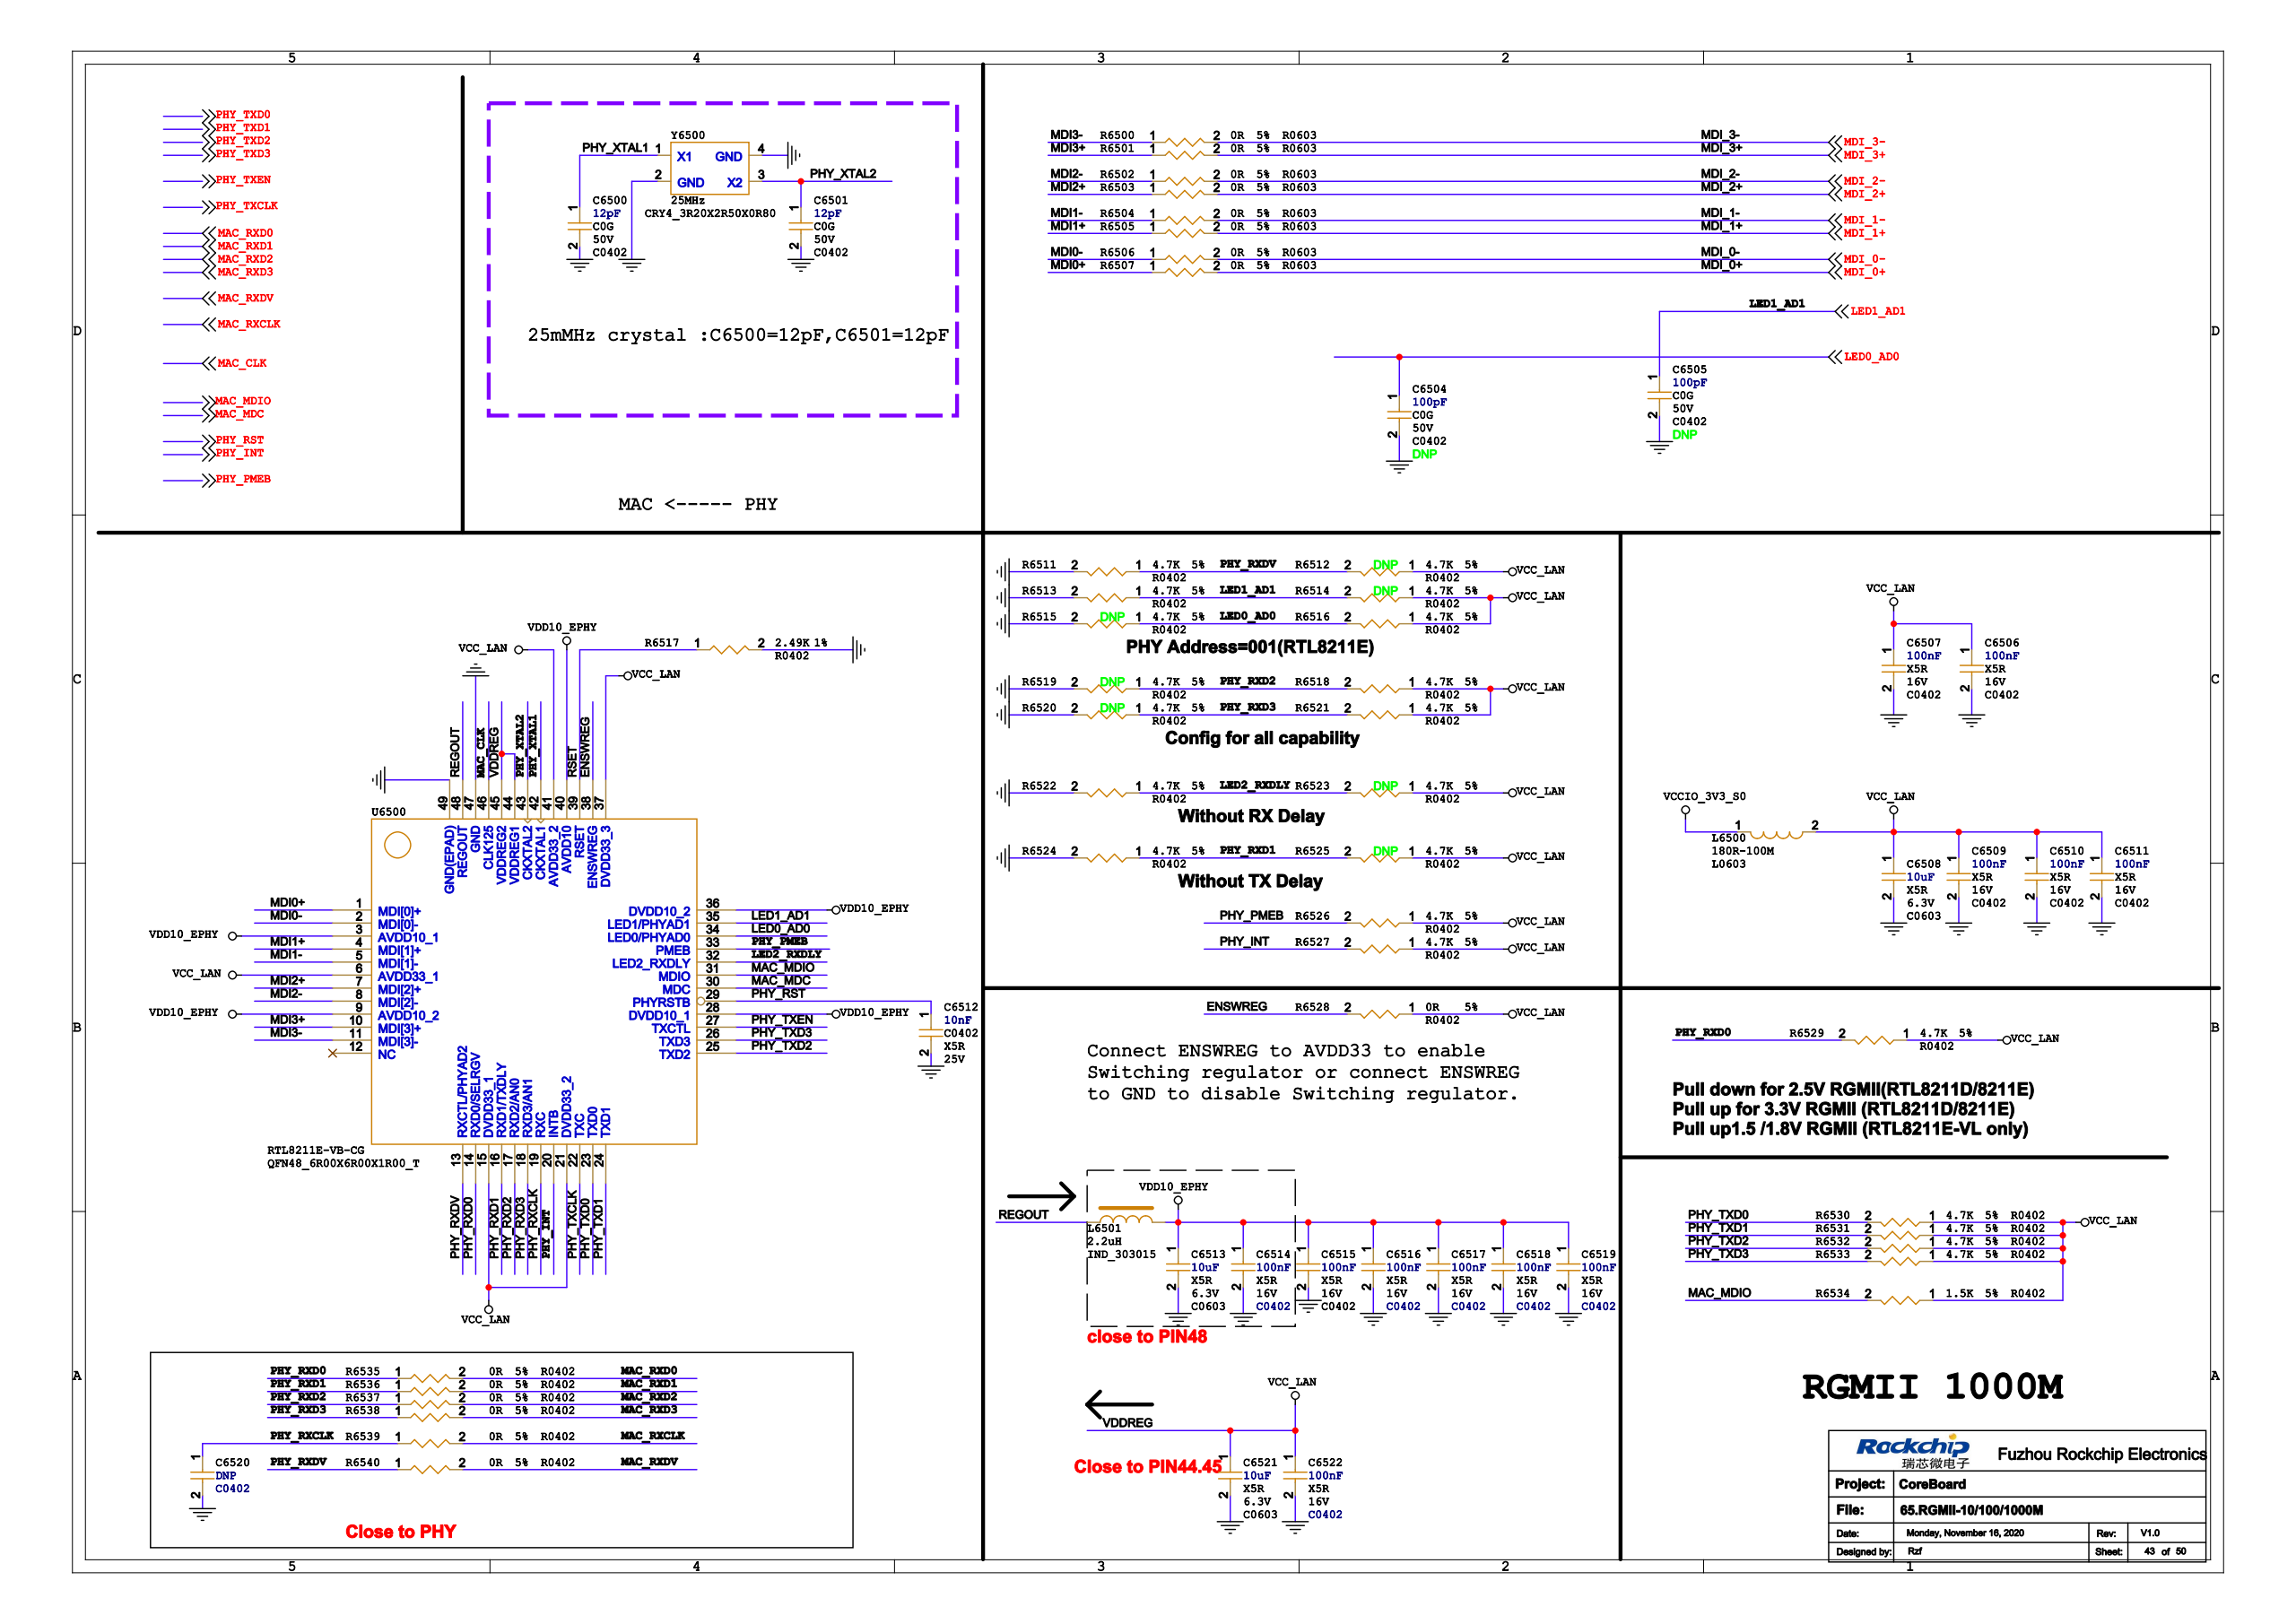Circuit board | Cadence Allegro | 749 parts | 717 nets | one sheet of the schematic
Parts on this sheet (reference | value | footprint):
C6500 | 12pF | C0402
C6501 | 12pF | C0402
C6504 | 100pF | C0402
C6505 | 100pF | C0402
C6506 | 100nF | C0402
C6507 | 100nF | C0402
C6508 | 10uF | C0603
C6509 | 100nF | C0402
C6510 | 100nF | C0402
C6511 | 100nF | C0402
C6512 | 10nF | C0402
C6513 | 10uF | C0603
C6514 | 100nF | C0402
C6515 | 100nF | C0402
C6516 | 100nF | C0402
C6517 | 100nF | C0402
C6518 | 100nF | C0402
C6519 | 100nF | C0402
C6520 | DNP | C0402
C6521 | 10uF | C0603
C6522 | 100nF | C0402
L6500 | 180R-100M | L0603
L6501 | 2.2uH | IND_303015
R6500 | 0R | R0603
R6501 | 0R | R0603
R6502 | 0R | R0603
R6503 | 0R | R0603
R6504 | 0R | R0603
R6505 | 0R | R0603
R6506 | 0R | R0603
R6507 | 0R | R0603
R6511 | 4.7K | R0402
R6512 | 4.7K | R0402
R6513 | 4.7K | R0402
R6514 | 4.7K | R0402
R6515 | 4.7K | R0402
R6516 | 4.7K | R0402
R6517 | 2.49K | R0402
R6518 | 4.7K | R0402
R6519 | 4.7K | R0402
R6520 | 4.7K | R0402
R6521 | 4.7K | R0402
R6522 | 4.7K | R0402
R6523 | 4.7K | R0402
R6524 | 4.7K | R0402
R6525 | 4.7K | R0402
R6526 | 4.7K | R0402
R6527 | 4.7K | R0402
R6528 | 0R | R0402
R6529 | 4.7K | R0402
R6530 | 4.7K | R0402
R6531 | 4.7K | R0402
R6532 | 4.7K | R0402
R6533 | 4.7K | R0402
R6534 | 1.5K | R0402
R6535 | 0R | R0402
R6536 | 0R | R0402
R6537 | 0R | R0402
R6538 | 0R | R0402
R6539 | 0R | R0402
R6540 | 0R | R0402
U6500 | RTL8211E-VB-CG | QFN48_6R00X6R00X1R00_T
Y6500 | 25MHz | CRY4_3R20X2R50X0R80
Nets of these parts (net: part-pin ...):
GND: C6500-2 C6501-2 C6504-2 C6505-2 C6506-2 C6507-2 C6508-2 C6509-2 C6510-2 C6511-2 C6512-2 C6513-2 C6514-2 C6515-2 C6516-2 C6517-2 C6518-2 C6519-2 C6520-2 C6521-2 C6522-2 R6511-2 R6513-2 R6515-2 R6517-2 R6519-2 R6520-2 R6522-2 R6524-2 Y6500-2 Y6500-4 U6500-47 U6500-49
PHY_XTAL1: C6500-1 Y6500-1 U6500-42
PHY_XTAL2: C6501-1 Y6500-3 U6500-43
PHY_RST: C6512-1 U6500-29
LED0_AD0: C6504-1 R6515-1 R6516-2 U6500-34
VCC_LAN: C6506-1 C6507-1 C6508-1 C6509-1 C6510-1 C6511-1 C6521-1 C6522-1 L6500-2 R6512-1 R6514-1 R6516-1 R6518-1 R6521-1 R6523-1 R6525-1 R6526-1 R6527-1 R6528-1 R6529-1 R6530-1 R6531-1 R6532-1 R6533-1 R6534-1 U6500-6 U6500-15 U6500-21 U6500-37 U6500-41 U6500-44 U6500-45
LED1_AD1: C6505-1 R6513-1 R6514-2 U6500-35
MDI_3-: R6500-2
MDI_3+: R6501-2
MDI_2-: R6502-2
MDI_2+: R6503-2
MDI_1-: R6504-2
MDI_1+: R6505-2
MDI_0-: R6506-2
MDI_0+: R6507-2
VCCIO_3V3_S0: L6500-1
REGOUT: L6501-1 U6500-48
VDD10_EPHY: C6513-1 C6514-1 C6515-1 C6516-1 C6517-1 C6518-1 C6519-1 L6501-2 U6500-3 U6500-9 U6500-28 U6500-36 U6500-40
RSET: R6517-1 U6500-39
MAC_CLK: U6500-46
ENSWREG: R6528-2 U6500-38
PHY_INT: R6527-2 U6500-20
LED2_RXDLY: R6522-1 R6523-2 U6500-32
MAC_MDC: U6500-30
MAC_MDIO: R6534-2 U6500-31
MDI0+: R6507-1 U6500-1
MDI0-: R6506-1 U6500-2
MDI1+: R6505-1 U6500-4
MDI1-: R6504-1 U6500-5
MDI2+: R6503-1 U6500-7
MDI2-: R6502-1 U6500-8
MDI3+: R6501-1 U6500-10
MDI3-: R6500-1 U6500-11
PHY_PMEB: R6526-2 U6500-33
PHY_RXCLK: C6520-1 R6539-1 U6500-19
PHY_RXDV: R6511-1 R6512-2 R6540-1 U6500-13
PHY_RXD0: R6529-2 R6535-1 U6500-14
PHY_RXD1: R6524-1 R6525-2 R6536-1 U6500-16
PHY_RXD2: R6518-2 R6519-1 R6537-1 U6500-17
PHY_RXD3: R6520-1 R6521-2 R6538-1 U6500-18
PHY_TXCLK: U6500-22
PHY_TXEN: U6500-27
PHY_TXD0: R6530-2 U6500-23
PHY_TXD1: R6531-2 U6500-24
PHY_TXD2: R6532-2 U6500-25
PHY_TXD3: R6533-2 U6500-26
MAC_RXCLK: R6539-2
MAC_RXD0: R6535-2
MAC_RXD1: R6536-2
MAC_RXD2: R6537-2
MAC_RXD3: R6538-2
MAC_RXDV: R6540-2